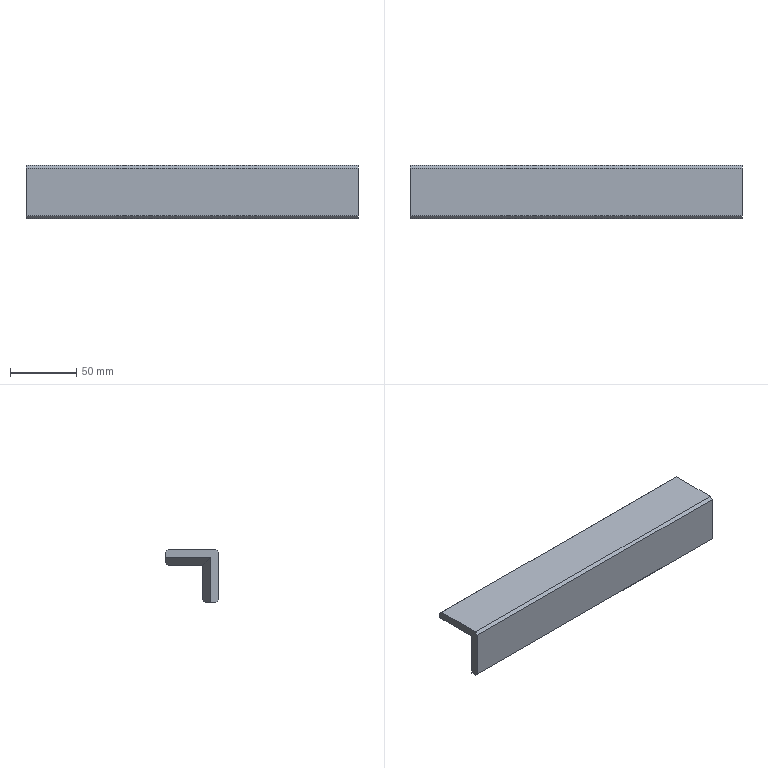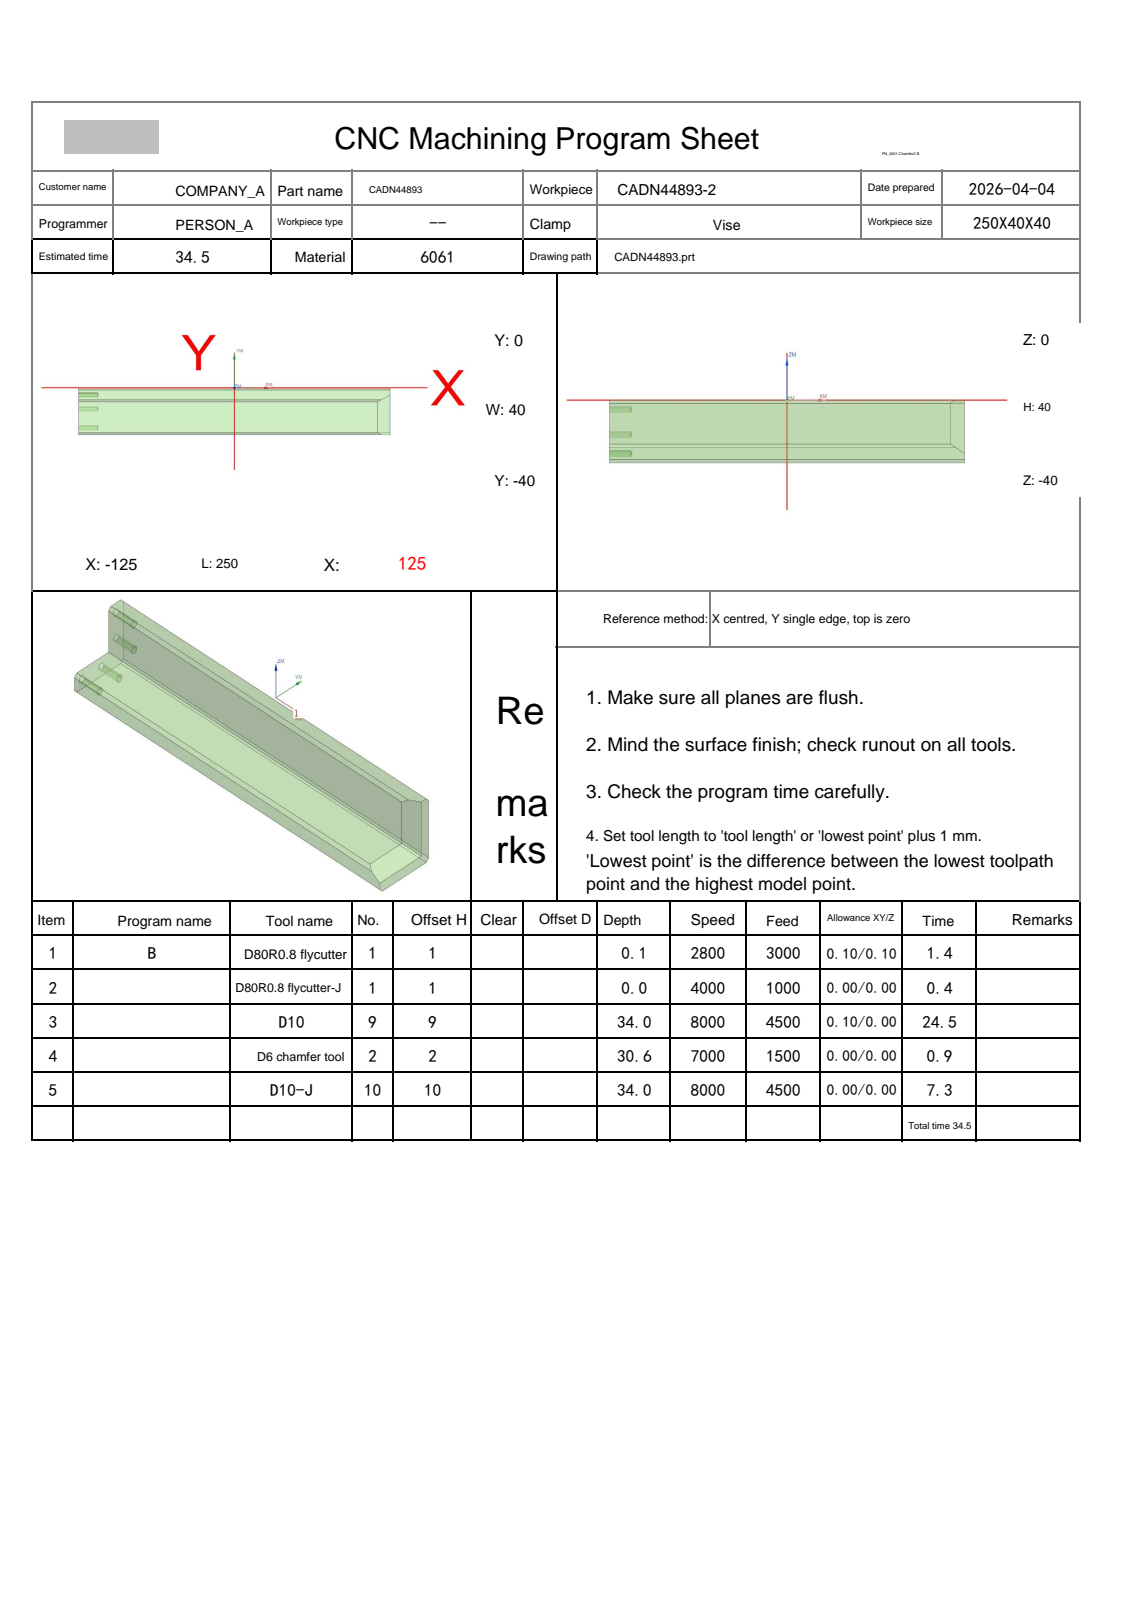NC program | NX | posted by the shop | part box 250 x 40 x 40 mm
Lines 1 to 108 of 8932:
%
O0001
(Machine time: 35.45 MIN)
(===Total Tool:4===)
(T1=D80R0.8 flycutter D=80.  R=0.8  D-  H01 Z=0.    )
(T9=D10     D=10.  R=0.   D-  H09 Z=-34.  )
(T2=D6 chamfer tool   D=6.   R=0.   D-  H02 Z=-30.6 )
(T10=D10-J  D=10.  R=0.   D10 H10 Z=-34.  )
G80 G90 G17 G49 G40
G91 G28 Z0
M01
N1 T01 M06
(D80R0.8 flycutter D=80. R=0.8 H=01 ce=0.10 di=0.10)
G00 G90 G54 X-177.097 Y-20. M03 S2800
G43 H01 Z50.
M08
Z6.011
G01 Z4.011 F3000.
X-165.097
X165.097
X177.097
Z6.011
G00 X-177.097
Z5.522
G01 Z3.522
X-165.097
X165.097
X177.097
Z5.522
G00 X-177.097
Z5.033
G01 Z3.033
X-165.097
X165.097
X177.097
Z5.033
G00 X-177.097
Z4.544
G01 Z2.544
X-165.097
X165.097
X177.097
Z4.544
G00 Z50.
X-177.097
Z4.056
G01 Z2.056
X-165.097
X165.097
X177.097
Z4.056
G00 Z50.
X-177.097
Z3.567
G01 Z1.567
X-165.097
X165.097
X177.097
Z3.567
G00 Z50.
X-177.097
Z3.078
G01 Z1.078
X-165.097
X165.097
X177.097
Z3.078
G00 Z50.
X-177.097
Z2.589
G01 Z.589
X-165.097
X165.097
X177.097
Z2.589
G00 Z50.
X-177.097
Z2.1
G01 Z.1
X-165.097
X165.097
X177.097
Z2.1
G00 Z50.
G91 G28 Z0.0
M05
M09
G91 G28 Z0.0
M01
N2 T01 M06
(D80R0.8 flycutter-J D=80. R=0.8 H=01 ce=0.00 di=0.00)
G00 G90 G54 X-176.999 Y-20. M03 S4000
G43 H01 Z50.
M08
Z2.
G01 Z0.0 F1000.
X-164.999
X164.999
X176.999
Z2.
G00 Z50.
G91 G28 Z0.0
M05
M09
G91 G28 Z0.0
M01